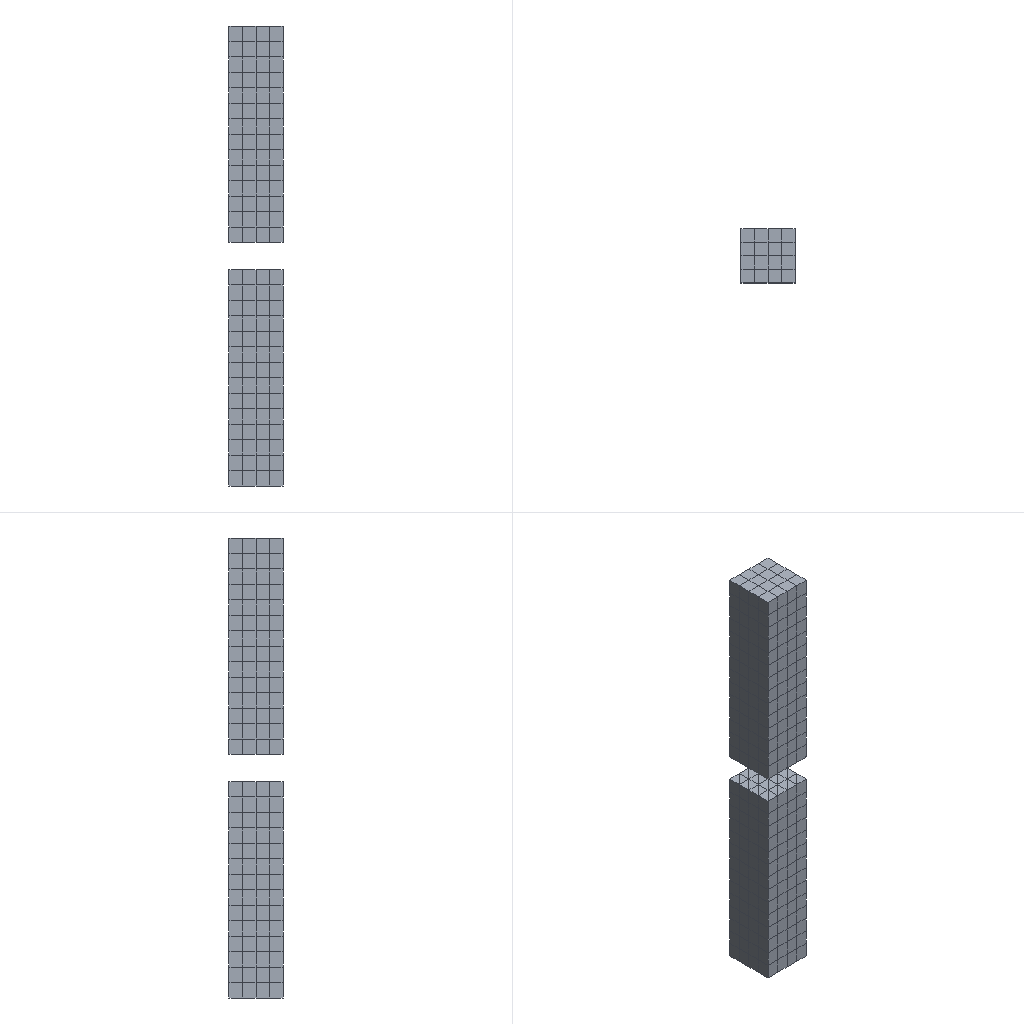Simulation study | ansys workbench
Ansys APDL input file, long lists of numbers shortened:
/batch
/config,noeldb,1     ! force off writing results to database
*get,_wallstrt,active,,time,wall
! ANSYS input file written by Workbench version 16.0 RELEASE
! File used for geometry attach: C:\Users\USE\AppData\Local\Temp\WB_LAPTOP-92PEKBNI_hmm_2756_2\unsaved_project_files\dp0\SYS\DM\SYS.agdb
/title,unsaved_project--Transient (A5)
*DIM,_wb_ProjectScratch_dir,string,248
_wb_ProjectScratch_dir(1) = 'C:\Users\USE\AppData\Local\Temp\WB_LAPTOP-92PEKBNI_hmm_2756_2\_ProjectScratch\Scr9FDD\'
*DIM,_wb_SolverFiles_dir,string,248
_wb_SolverFiles_dir(1) = 'C:\Users\USE\AppData\Local\Temp\WB_LAPTOP-92PEKBNI_hmm_2756_2\unsaved_project_files\dp0\SYS\MECH\'
*DIM,_wb_userfiles_dir,string,248
_wb_userfiles_dir(1) = 'C:\Users\USE\AppData\Local\Temp\WB_LAPTOP-92PEKBNI_hmm_2756_2\unsaved_project_files\user_files\'
/com,--- Data in consistent NMM units. See Solving Units in the help system for more information.
/units,MPA
/nopr
/wb,file,start              !  signify a WB generated input file
/prep7
! Turn off shape checking because checks already performed inside WB mesher.
! See help system for more information.
SHPP,OFF,,NOWARN
/nolist
etcon,set             ! allow ANSYS to choose best KEYOP's for 180x elements
/com,*********** Nodes for the whole assembly ***********
nblock,3
(1i9,3e20.9e3)
        1   -2.500000000E+000    2.500000000E+000   -4.214285714E+001
! (2649 more lines like these left out)
-1
/wb,elem,start            !  set before creation of elements
/com,*********** Elements for Body 1 "Solid" ***********
et,1,186
keyo,1,2,1          ! set full integration on SOLID186
eblock,19,solid,,224
(19i9)
        1        1        1        1        0        0        0        0       20        0      225     1326     1691     1611     1595     1481     1700     1612     1608
! (447 more lines like these left out)
-1
/com,*********** Elements for Body 2 "Solid" ***********
et,2,186
keyo,2,2,1          ! set full integration on SOLID186
eblock,19,solid,,224
(19i9)
        2        2        2        2        0        0        0        0       20        0        1        1      354      290      232      156      363      291      271
! (447 more lines like these left out)
-1
/wb,elem,end               !  done creating elements
/com,*********** Send User Defined Coordinate System(s) ***********
csys,0
toffst,273.15,  ! Temperature offset from absolute zero
/com,*********** Set Reference Temperature ***********
tref,22.
/wb,mat,start              !  starting to send materials
/com,*********** Send Materials ***********
MP,DENS,1,7.85e-09,	! tonne mm^-3
MP,ALPX,1,1.2e-05,	! C^-1
MP,C,1,434000000,	! mm^2 s^-2 C^-1
MP,KXX,1,60.5,	! tonne mm s^-3 C^-1
MP,RSVX,1,0.00017,	! ohm mm
MP,EX,1,200000,	! tonne s^-2 mm^-1
MP,NUXY,1,0.3,
MP,MURX,1,10000,
MP,DENS,2,7.85e-09,	! tonne mm^-3
MP,ALPX,2,1.2e-05,	! C^-1
MP,C,2,434000000,	! mm^2 s^-2 C^-1
MP,KXX,2,60.5,	! tonne mm s^-3 C^-1
MP,RSVX,2,0.00017,	! ohm mm
MP,EX,2,200000,	! tonne s^-2 mm^-1
MP,NUXY,2,0.3,
MP,MURX,2,10000,
/wb,mat,end                !  done sending materials
!************************* Model Summary ********************
!Solid,	Structural Steel,	matid,	1
!Solid,	Structural Steel,	matid,	2
!************************* End Model Summary ********************
! get the diagonal of the bounding box. Needed later for other things
*get,_xmin,node,,mnloc,x
*get,_ymin,node,,mnloc,y
*get,_zmin,node,,mnloc,z
*get,_xmax,node,,mxloc,x
*get,_ymax,node,,mxloc,y
*get,_zmax,node,,mxloc,z
_ASMDIAG=(_xmax-_xmin)*(_xmax-_xmin)+(_ymax-_ymin)*(_ymax-_ymin)+(_zmax-_zmin)*(_zmax-_zmin)
_ASMDIAG=SQRT(_ASMDIAG)
/wb,contact,start          !  starting to send contact
/com,*********** Create Contact "Frictional - Solid To Solid" ***********
/com,            Real Constant Set For Above Contact Is 4 & 3
*set,tid,4
*set,cid,3
r,tid
r,cid
et,tid,170
et,cid,174
eblock,10,,,16
(15i9)
      449        4        4        4        0     1670     1689     1698     1669     2606     2636     2604     2603
! (15 more lines like these left out)
-1
eblock,10,,,16
(15i9)
      465        3        3        3        0     1670     1689     1698     1669     2606     2636     2604     2603
! (15 more lines like these left out)
-1
eblock,10,,,16
(15i9)
      481        3        4        3        0      347      364      196      202     1284     1004     1003     1017
! (15 more lines like these left out)
-1
eblock,10,,,16
(15i9)
      497        4        3        4        0      347      364      196      202     1284     1004     1003     1017
! (15 more lines like these left out)
-1
keyo,cid,8,2               ! auto create asymmetric contact (from Program Controlled setting)
keyo,cid,10,2              ! adjust contact stiffness each NR iteration (from Program Controlled setting)
keyo,cid,12,0              ! standard contact
mp,mu,cid,0.1	! unitless
keyo,cid,2,0               ! augmented Lagrange (from Program Controlled setting)
keyo,cid,4,0               ! on Gauss point (from Program Controlled setting)
keyo,cid,9,0               ! use real geometry with stepped effects
keyo,cid,7,0               ! No Prediction
rmod,tid,3,1.	! FKN
rmod,tid,5,0.	! ICONT
rmod,tid,6,0.	! PINB
rmod,tid,10,0.	! CNOF
rmod,tid,12,0.	! FKT
rmod,tid,36,32	! WB DSID
rmod,cid,3,1.	! FKN
rmod,cid,5,0.	! ICONT
rmod,cid,6,0.	! PINB
rmod,cid,10,0.	! CNOF
rmod,cid,12,0.	! FKT
rmod,cid,36,32	! WB DSID
nsel,all
esel,all
/wb,contact,end            !  done creating contacts
/golist
/wb,load,start             !  starting to send loads
/com,*********** Fixed Supports ***********
CMBLOCK,_FIXEDSU,NODE,       65
(8i10)
      1524      1525      1526      1541      1556      1613      1614      1615
! (8 more lines like these left out)
cmsel,s,_FIXEDSU
d,all,all
nsel,all
/com,******* Constant Zero Displacement X *******
CMBLOCK,_DISPZEROUX,NODE,       65
(8i10)
       196       197       198       202       217       284       285       286
! (8 more lines like these left out)
cmsel,s,_DISPZEROUX
d,all,ux,0
nsel,all
/com,******* Constant Zero Displacement Y *******
CMBLOCK,_DISPZEROUY,NODE,       65
(8i10)
       196       197       198       202       217       284       285       286
! (8 more lines like these left out)
cmsel,s,_DISPZEROUY
d,all,uy,0
nsel,all
nsel,all
/com,*********** Create Displacement Tables and Functions ******
*DIM,_loadvari37xp,TABLE,1,1,1,TIME,
! Time values
_loadvari37xp(1,0,1) = 1.
! Load values
_loadvari37xp(1,1,1) = 0.
*DIM,_loadvari37xn,TABLE,1,1,1,TIME,
! Time values
_loadvari37xn(1,0,1) = 1.
! Load values
_loadvari37xn(1,1,1) = -0.
*DIM,_loadvari37yp,TABLE,1,1,1,TIME,
! Time values
_loadvari37yp(1,0,1) = 1.
! Load values
_loadvari37yp(1,1,1) = 0.
*DIM,_loadvari37yn,TABLE,1,1,1,TIME,
! Time values
_loadvari37yn(1,0,1) = 1.
! Load values
_loadvari37yn(1,1,1) = -0.
*DIM,_loadvari37zp,TABLE,2,1,1,TIME,
! Time values
_loadvari37zp(1,0,1) = 0.
_loadvari37zp(2,0,1) = 1.
! Load values
_loadvari37zp(1,1,1) = 0.
_loadvari37zp(2,1,1) = 6.
*DIM,_loadvari37zn,TABLE,2,1,1,TIME,
! Time values
_loadvari37zn(1,0,1) = 0.
_loadvari37zn(2,0,1) = 1.
! Load values
_loadvari37zn(1,1,1) = -0.
_loadvari37zn(2,1,1) = -6.
/gst,on,on
fini
*get,_numnode,node,0,count
*get,_numelem,elem,0,count
*get, _MAXELEMNUM, elem, 0, NUM, MAX
*get, _MAXNODENUM, node, 0, NUM, MAX
*get, _MAXELEMTYPE, etyp, 0, NUM, MAX
*get, _MAXREALCONST, real, 0, NUM, MAX
/go
/wb,load,end               !  done creating loads
/com,--- Number of total nodes = %_numnode%
/com,--- Number of contact elements = 64
/com,--- Number of spring elements = 0
/com,--- Number of bearing elements = 0
/com,--- Number of solid elements = 448
/com,--- Number of total elements = %_numelem%
*get,_wallbsol,active,,time,wall
/com,****************************************************************************
/com,*************************    SOLUTION       ********************************
/com,****************************************************************************
/solu
antype,4                   ! transient analysis
nlgeom,on                  ! Turn on Large Deformation Effects
kbc,1                      ! stepped BC's
eqsl,pcg,1e-8,,,,,,1
cntr,print,1               ! print out contact info and also make no initial contact an error
trnopt,full,,,,,hht        ! HHT time integration method
tintp,0.1	! Numerical Damping
nldiag,cont,iter           ! print out contact info each equilibrium iteration
resc,define,last,last,,dele	   ! Program Controlled
/com,****************************************************
/com,******************* SOLVE FOR LS 1 ****************
/com,*** Set Displacements ***
CMBLOCK,_CM37UZ_ZP,NODE,       65
(8i10)
       196       197       198       202       217       284       285       286
! (8 more lines like these left out)
cmsel,s,_CM37UZ_ZP
d,all,uz,%_loadvari37zp%
nsel,all
/nopr
/gopr
autots,on                   ! User turned on automatic time stepping
deltim,0.1,0.1,0.1,OFF
time,1.
timint,on                  ! Turn on time integration effects
outres,erase
outres,all,none
outres,nsol,all
outres,rsol,all
outres,strs,all
outres,epel,all
outres,eppl,all
outres,v,all
outres,a,all
stabilize,off                   ! Stabilization turned OFF by user
! *********** WB SOLVE COMMAND ***********
! check interactive state
*get,ANSINTER_,active,,int
*if,ANSINTER_,ne,0,then
/eof
*endif
solve
/com *************** Write FE CONNECTORS *********
CEWRITE,file,ce,,INTE
/com,****************************************************
/com,*************** FINISHED SOLVE FOR LS 1 *************
*set,_DS_PROGRESS          ! turn off progress updates to avoid virus scanning bug
*get,_wallasol,active,,time,wall
/nopr
*get,_numnode,node,0,count
*get,_numelem,elem,0,count
*get, _MAXELEMNUM, elem, 0, NUM, MAX
*get, _MAXNODENUM, node, 0, NUM, MAX,,,INTERNAL
*get, _MAXELEMTYPE, etyp, 0, NUM, MAX
*get, _MAXREALCONST, real, 0, NUM, MAX
/gopr
*get,_PCGITER,active,,solu,cgiter
/post1
xmlo,ENCODING,ISO-8859-1
xmlo,parm
/xml,parm,xml
fini
/gopr
*get,_walldone,active,,time,wall
_preptime=(_wallbsol-_wallstrt)*3600
_solvtime=(_wallasol-_wallbsol)*3600
_posttime=(_walldone-_wallasol)*3600
_totaltim=(_walldone-_wallstrt)*3600
/wb,file,end               ! done with WB generated input